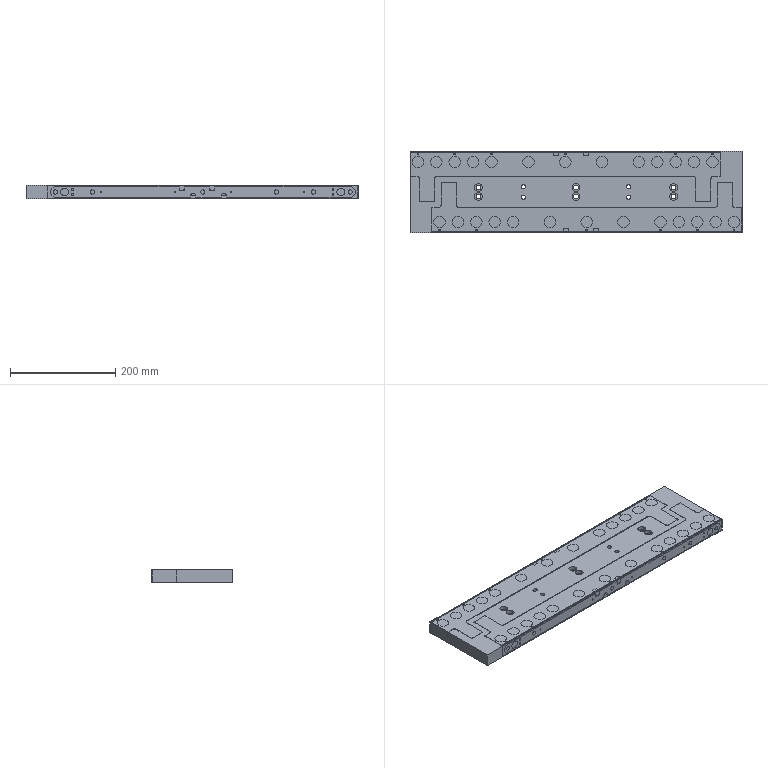NC program | NX | posted with a generic post | part box 631 x 154 x 25 mm
Lines 1 to 130 of 18383:
N10 G17 G21 G94 G90
(FLOOR_WALL , TOOL : D63)
N12 T01 M6
N14 G54
N16 G17 G0 G90 X-253. Y69.997 B0. C0. S6500 M3
N18 G43 Z30. H1
N20 Z3.
N22 G94 G1 Z0. F1250.
N24 X-250.
N26 X450.
N28 Y25.065
N30 X-250.
N32 Y-19.868
N34 X450.
N36 Y-64.8
N38 X-250.
N40 X-253.
N42 Z3.
N44 G0 Z30.
N46 M5
(DRILLING_COPY_1 , TOOL : D6A45)
N48 T07 M6
N50 G54
N52 G17 G0 G90 X-159.5 Y-82. B0. C0. S3000 M3
N54 G43 Z30. H7
N56 G94 G81 G98 Z-2.1 F200. R3.
N58 Y-67.
N60 X-124.5
N62 X-89.5
N64 Y-82.
N66 X-54.5 Y-67.
N68 X-19.5
N70 X50.5
N72 X120.5
N74 Y-82.
N76 X190.5 Y-67.
N78 X260.5 Y-82.
N80 Y-67.
N82 X295.5
N84 X330.5
N86 Y-82.
N88 X365.5 Y-67.
N90 X400.5 Y-82.
N92 Y-67.
N94 X359.5 Y47.
N96 Y62.
N98 X324.5 Y47.
N100 X289.5 Y62.
N102 Y47.
N104 X254.5
N106 X219.5
N108 X149.5
N110 X79.5
N112 Y62.
N114 X9.5 Y47.
N116 X-60.5 Y62.
N118 Y47.
N120 X-95.5
N122 X-130.5 Y62.
N124 Y47.
N126 X-165.5
N128 X-200.5
N130 Y62.
N132 G80
N134 G0 X-200.5 Y62. Z30.
N136 M5
(DRILLING_COPY_2 , TOOL : 3.3ZT)
N138 T13 M6
N140 G54
N142 G17 G0 G90 X-89.5 Y-82. B0. C0. S2000 M3
N144 G43 Z30. H13
N146 G94 G83 G98 Z-26.991 F100. Q2. R3.
N148 X-159.5
N150 X-200.5 Y62.
N152 X-130.5
N154 X-60.5
N156 X79.5
N158 X120.5 Y-82.
N160 X260.5
N162 X330.5
N164 X400.5
N166 X359.5 Y62.
N168 X289.5
N170 G80
N172 G0 X289.5 Y62. Z30.
N174 M5
(DRILLING_COPY_2_COPY , TOOL : 15.5ZT)
N176 T16 M6
N178 G54
N180 G17 G0 G90 X-159.5 Y-67. B0. C0. S1000 M3
N182 G43 Z30. H16
N184 G94 G83 G98 Z-30.307 F200. Q4. R3.
N186 X-124.5
N188 X-89.5
N190 X-54.5
N192 X-19.5
N194 X50.5
N196 X120.5
N198 X190.5
N200 X260.5
N202 X295.5
N204 X330.5
N206 X365.5
N208 X400.5
N210 X359.5 Y47.
N212 X324.5
N214 X289.5
N216 X254.5
N218 X219.5
N220 X149.5
N222 X79.5
N224 X9.5
N226 X-60.5
N228 X-95.5
N230 X-130.5
N232 X-165.5
N234 X-200.5
N236 G80
N238 G0 X-200.5 Y47. Z30.
N240 M5